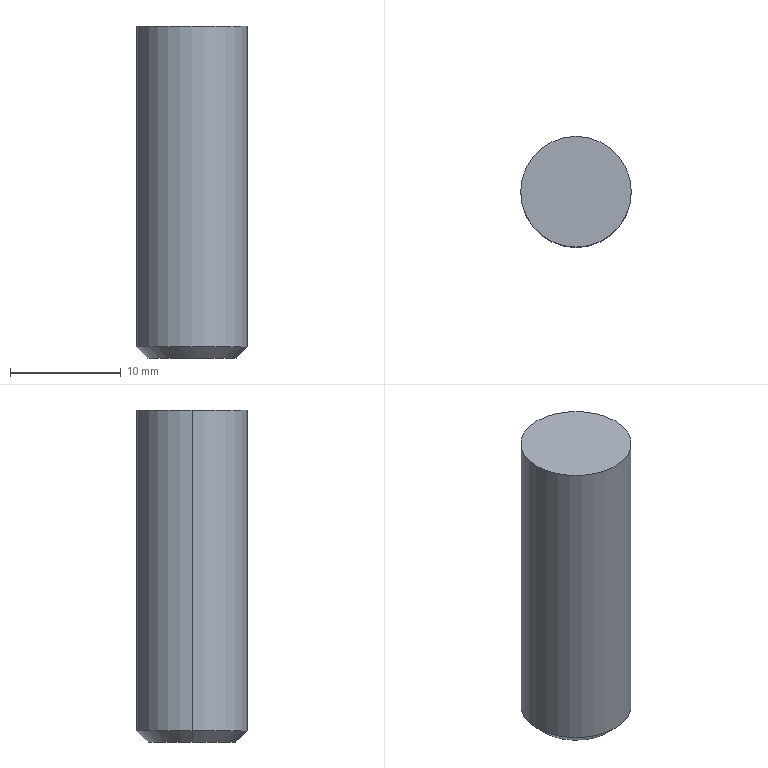Part | SolidWorks | features Chamfer 1, Extrusion 1 | 1 solid | 6 faces | box 10 x 10 x 30 mm | volume 2342 mm3 | cone 2 | cylinder 2 | plane 2 | commonest cylinder face diameters 10 x2
STEP:
#1=CARTESIAN_POINT('',(-4.,0.,0.));
#2=VERTEX_POINT('',#1);
#3=CARTESIAN_POINT('',(4.,0.,0.));
#4=VERTEX_POINT('',#3);
#5=CARTESIAN_POINT('',(0.,0.,0.));
#6=DIRECTION('',(0.,0.,-1.));
#7=DIRECTION('',(1.,0.,0.));
#8=AXIS2_PLACEMENT_3D('',#5,#6,#7);
#9=CIRCLE('',#8,4.);
#10=EDGE_CURVE('',#2,#4,#9,.T.);
#11=ORIENTED_EDGE('',*,*,#10,.F.);
#12=CARTESIAN_POINT('',(-5.,0.,1.));
#13=VERTEX_POINT('',#12);
#14=CARTESIAN_POINT('',(-5.,0.,1.));
#15=DIRECTION('',(-0.7071,0.,0.7071));
#16=VECTOR('',#15,1000.);
#17=LINE('',#14,#16);
#18=EDGE_CURVE('',#2,#13,#17,.T.);
#19=ORIENTED_EDGE('',*,*,#18,.T.);
#20=CARTESIAN_POINT('',(5.,0.,1.));
#21=VERTEX_POINT('',#20);
#22=CARTESIAN_POINT('',(0.,0.,1.));
#23=DIRECTION('',(0.,0.,1.));
#24=DIRECTION('',(1.,0.,0.));
#25=AXIS2_PLACEMENT_3D('',#22,#23,#24);
#26=CIRCLE('',#25,5.);
#27=EDGE_CURVE('',#21,#13,#26,.T.);
#28=ORIENTED_EDGE('',*,*,#27,.F.);
#29=CARTESIAN_POINT('',(5.,0.,1.));
#30=DIRECTION('',(0.7071,0.,0.7071));
#31=VECTOR('',#30,1000.);
#32=LINE('',#29,#31);
#33=EDGE_CURVE('',#4,#21,#32,.T.);
#34=ORIENTED_EDGE('',*,*,#33,.F.);
#35=EDGE_LOOP('',(#11,#19,#28,#34));
#36=FACE_OUTER_BOUND('',#35,.T.);
#37=CARTESIAN_POINT('',(0.,0.,1.));
#38=DIRECTION('',(0.,0.,1.));
#39=DIRECTION('',(1.,0.,0.));
#40=AXIS2_PLACEMENT_3D('',#37,#38,#39);
#41=CONICAL_SURFACE('',#40,5.,0.7854);
#42=ADVANCED_FACE('',(#36),#41,.T.);
#43=CARTESIAN_POINT('',(5.,0.,30.));
#44=VERTEX_POINT('',#43);
#45=CARTESIAN_POINT('',(-5.,0.,30.));
#46=VERTEX_POINT('',#45);
#47=CARTESIAN_POINT('',(0.,0.,30.));
#48=DIRECTION('',(0.,0.,1.));
#49=DIRECTION('',(1.,0.,0.));
#50=AXIS2_PLACEMENT_3D('',#47,#48,#49);
#51=CIRCLE('',#50,5.);
#52=EDGE_CURVE('',#44,#46,#51,.T.);
#53=ORIENTED_EDGE('',*,*,#52,.F.);
#54=CARTESIAN_POINT('',(5.,0.,30.));
#55=DIRECTION('',(0.,0.,-1.));
#56=VECTOR('',#55,1000.);
#57=LINE('',#54,#56);
#58=EDGE_CURVE('',#44,#21,#57,.T.);
#59=ORIENTED_EDGE('',*,*,#58,.T.);
#60=ORIENTED_EDGE('',*,*,#27,.T.);
#61=CARTESIAN_POINT('',(-5.,0.,30.));
#62=DIRECTION('',(0.,0.,-1.));
#63=VECTOR('',#62,1000.);
#64=LINE('',#61,#63);
#65=EDGE_CURVE('',#46,#13,#64,.T.);
#66=ORIENTED_EDGE('',*,*,#65,.F.);
#67=EDGE_LOOP('',(#53,#59,#60,#66));
#68=FACE_OUTER_BOUND('',#67,.T.);
#69=CARTESIAN_POINT('',(0.,0.,30.));
#70=DIRECTION('',(0.,0.,-1.));
#71=DIRECTION('',(-1.,0.,0.));
#72=AXIS2_PLACEMENT_3D('',#69,#70,#71);
#73=CYLINDRICAL_SURFACE('',#72,5.);
#74=ADVANCED_FACE('',(#68),#73,.T.);
#75=ORIENTED_EDGE('',*,*,#58,.F.);
#76=CARTESIAN_POINT('',(0.,0.,30.));
#77=DIRECTION('',(0.,0.,1.));
#78=DIRECTION('',(1.,0.,0.));
#79=AXIS2_PLACEMENT_3D('',#76,#77,#78);
#80=CIRCLE('',#79,5.);
#81=EDGE_CURVE('',#46,#44,#80,.T.);
#82=ORIENTED_EDGE('',*,*,#81,.F.);
#83=ORIENTED_EDGE('',*,*,#65,.T.);
#84=CARTESIAN_POINT('',(0.,0.,1.));
#85=DIRECTION('',(0.,0.,1.));
#86=DIRECTION('',(1.,0.,0.));
#87=AXIS2_PLACEMENT_3D('',#84,#85,#86);
#88=CIRCLE('',#87,5.);
#89=EDGE_CURVE('',#13,#21,#88,.T.);
#90=ORIENTED_EDGE('',*,*,#89,.T.);
#91=EDGE_LOOP('',(#75,#82,#83,#90));
#92=FACE_OUTER_BOUND('',#91,.T.);
#93=CARTESIAN_POINT('',(0.,0.,30.));
#94=DIRECTION('',(0.,0.,-1.));
#95=DIRECTION('',(-1.,0.,0.));
#96=AXIS2_PLACEMENT_3D('',#93,#94,#95);
#97=CYLINDRICAL_SURFACE('',#96,5.);
#98=ADVANCED_FACE('',(#92),#97,.T.);
#99=ORIENTED_EDGE('',*,*,#81,.T.);
#100=ORIENTED_EDGE('',*,*,#52,.T.);
#101=EDGE_LOOP('',(#99,#100));
#102=FACE_OUTER_BOUND('',#101,.T.);
#103=CARTESIAN_POINT('',(0.,0.,30.));
#104=DIRECTION('',(0.,0.,1.));
#105=DIRECTION('',(1.,0.,0.));
#106=AXIS2_PLACEMENT_3D('',#103,#104,#105);
#107=PLANE('',#106);
#108=ADVANCED_FACE('',(#102),#107,.T.);
#109=CARTESIAN_POINT('',(0.,0.,0.));
#110=DIRECTION('',(0.,0.,-1.));
#111=DIRECTION('',(1.,0.,0.));
#112=AXIS2_PLACEMENT_3D('',#109,#110,#111);
#113=CIRCLE('',#112,4.);
#114=EDGE_CURVE('',#4,#2,#113,.T.);
#115=ORIENTED_EDGE('',*,*,#114,.T.);
#116=ORIENTED_EDGE('',*,*,#10,.T.);
#117=EDGE_LOOP('',(#115,#116));
#118=FACE_OUTER_BOUND('',#117,.T.);
#119=CARTESIAN_POINT('',(0.,0.,0.));
#120=DIRECTION('',(0.,0.,1.));
#121=DIRECTION('',(1.,0.,0.));
#122=AXIS2_PLACEMENT_3D('',#119,#120,#121);
#123=PLANE('',#122);
#124=ADVANCED_FACE('',(#118),#123,.F.);
#125=ORIENTED_EDGE('',*,*,#18,.F.);
#126=ORIENTED_EDGE('',*,*,#114,.F.);
#127=ORIENTED_EDGE('',*,*,#33,.T.);
#128=ORIENTED_EDGE('',*,*,#89,.F.);
#129=EDGE_LOOP('',(#125,#126,#127,#128));
#130=FACE_OUTER_BOUND('',#129,.T.);
#131=CARTESIAN_POINT('',(0.,0.,1.));
#132=DIRECTION('',(0.,0.,1.));
#133=DIRECTION('',(1.,0.,0.));
#134=AXIS2_PLACEMENT_3D('',#131,#132,#133);
#135=CONICAL_SURFACE('',#134,5.,0.7854);
#136=ADVANCED_FACE('',(#130),#135,.T.);
#137=CLOSED_SHELL('',(#42,#74,#98,#108,#124,#136));
#138=MANIFOLD_SOLID_BREP('',#137);
#139=CARTESIAN_POINT('',(0.,0.,0.));
#140=DIRECTION('',(0.,0.,1.));
#141=DIRECTION('',(1.,0.,0.));
#142=AXIS2_PLACEMENT_3D('',#139,#140,#141);
#143=(LENGTH_UNIT()NAMED_UNIT(*)SI_UNIT(.MILLI.,.METRE.));
#144=UNCERTAINTY_MEASURE_WITH_UNIT(LENGTH_MEASURE(0.00001),#143,'','');
#145=(NAMED_UNIT(*)PLANE_ANGLE_UNIT()SI_UNIT($,.RADIAN.));
#146=(NAMED_UNIT(*)SI_UNIT($,.STERADIAN.)SOLID_ANGLE_UNIT());
#147=(GEOMETRIC_REPRESENTATION_CONTEXT(3)GLOBAL_UNCERTAINTY_ASSIGNED_CONTEXT((#144))GLOBAL_UNIT_ASSIGNED_CONTEXT((#143,#145,#146))REPRESENTATION_CONTEXT('',''));
#148=ADVANCED_BREP_SHAPE_REPRESENTATION('',(#138,#142),#147);